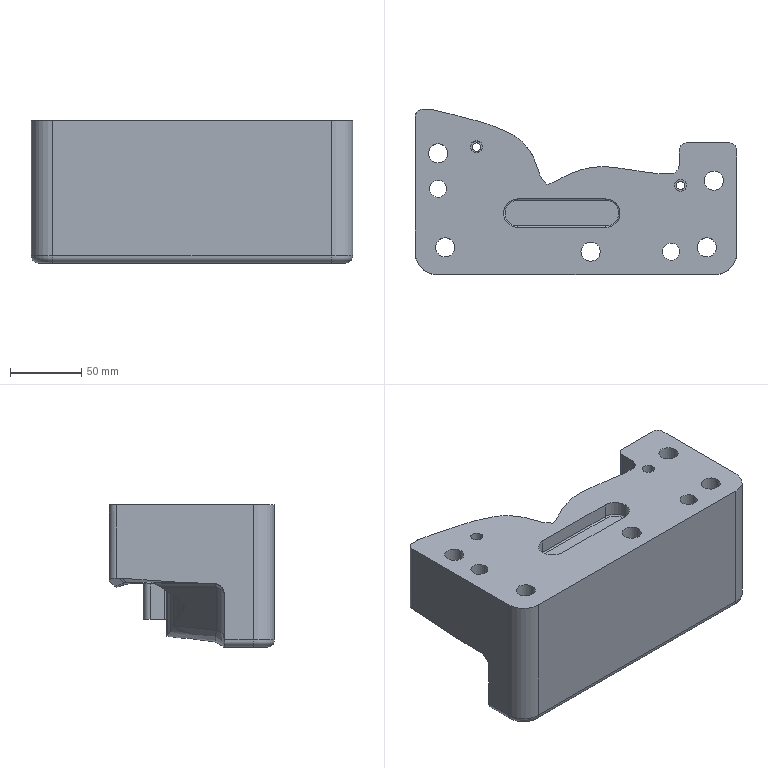Part | STEP file | lll_id3486_x_t | 1 solid | 154 faces | box 226 x 116.139 x 100 mm | volume 1449616 mm3 | plane 82 | cylinder 44 | spline 18 | torus 5 | other 3 | cone 2 | commonest cylinder face diameters 10 x7 13.509 x5 20.007 x5 14 x4 16 x3 30 x3